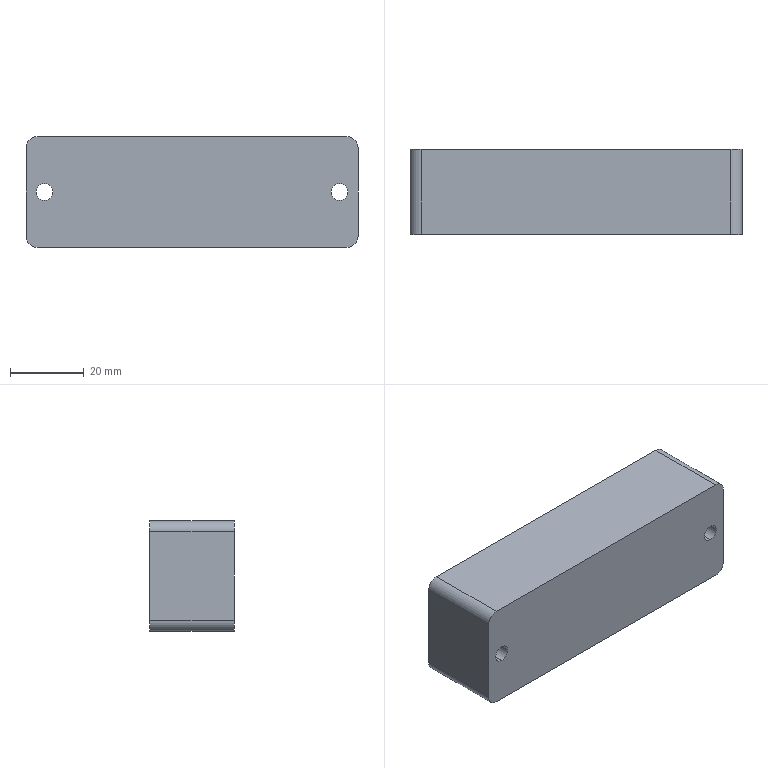Part | SolidWorks | features Extrusion 1, Fillet 1, HoleWzd 1 | 1 solid | 20 faces | box 90 x 23 x 30 mm | volume 60888 mm3 | cylinder 12 | plane 8 | commonest cylinder face diameters 4.5 x4 6 x4 8 x4
STEP:
#1=CARTESIAN_POINT('',(-40.,7.1,-4.));
#2=VERTEX_POINT('',#1);
#3=CARTESIAN_POINT('',(-40.,7.1,4.));
#4=VERTEX_POINT('',#3);
#5=CARTESIAN_POINT('',(-40.,7.1,0.));
#6=DIRECTION('',(0.,1.,0.));
#7=DIRECTION('',(0.,0.,1.));
#8=AXIS2_PLACEMENT_3D('',#5,#6,#7);
#9=CIRCLE('',#8,4.);
#10=EDGE_CURVE('',#2,#4,#9,.T.);
#11=ORIENTED_EDGE('',*,*,#10,.F.);
#12=CARTESIAN_POINT('',(-40.,11.5,-4.));
#13=VERTEX_POINT('',#12);
#14=CARTESIAN_POINT('',(-40.,11.5,-4.));
#15=DIRECTION('',(0.,1.,0.));
#16=VECTOR('',#15,1000.);
#17=LINE('',#14,#16);
#18=EDGE_CURVE('',#2,#13,#17,.T.);
#19=ORIENTED_EDGE('',*,*,#18,.T.);
#20=CARTESIAN_POINT('',(-40.,11.5,4.));
#21=VERTEX_POINT('',#20);
#22=CARTESIAN_POINT('',(-40.,11.5,0.));
#23=DIRECTION('',(0.,1.,0.));
#24=DIRECTION('',(0.,0.,1.));
#25=AXIS2_PLACEMENT_3D('',#22,#23,#24);
#26=CIRCLE('',#25,4.);
#27=EDGE_CURVE('',#13,#21,#26,.T.);
#28=ORIENTED_EDGE('',*,*,#27,.T.);
#29=CARTESIAN_POINT('',(-40.,11.5,4.));
#30=DIRECTION('',(0.,1.,0.));
#31=VECTOR('',#30,1000.);
#32=LINE('',#29,#31);
#33=EDGE_CURVE('',#4,#21,#32,.T.);
#34=ORIENTED_EDGE('',*,*,#33,.F.);
#35=EDGE_LOOP('',(#11,#19,#28,#34));
#36=FACE_OUTER_BOUND('',#35,.T.);
#37=CARTESIAN_POINT('',(-40.,11.5,0.));
#38=DIRECTION('',(0.,1.,0.));
#39=DIRECTION('',(0.,0.,1.));
#40=AXIS2_PLACEMENT_3D('',#37,#38,#39);
#41=CYLINDRICAL_SURFACE('',#40,4.);
#42=ADVANCED_FACE('',(#36),#41,.F.);
#43=CARTESIAN_POINT('',(-40.,-11.5,-2.25));
#44=VERTEX_POINT('',#43);
#45=CARTESIAN_POINT('',(-40.,-11.5,2.25));
#46=VERTEX_POINT('',#45);
#47=CARTESIAN_POINT('',(-40.,-11.5,0.));
#48=DIRECTION('',(0.,1.,0.));
#49=DIRECTION('',(0.,0.,1.));
#50=AXIS2_PLACEMENT_3D('',#47,#48,#49);
#51=CIRCLE('',#50,2.25);
#52=EDGE_CURVE('',#44,#46,#51,.T.);
#53=ORIENTED_EDGE('',*,*,#52,.F.);
#54=CARTESIAN_POINT('',(-40.,7.1,-2.25));
#55=VERTEX_POINT('',#54);
#56=CARTESIAN_POINT('',(-40.,11.5,-2.25));
#57=DIRECTION('',(0.,1.,0.));
#58=VECTOR('',#57,1000.);
#59=LINE('',#56,#58);
#60=EDGE_CURVE('',#44,#55,#59,.T.);
#61=ORIENTED_EDGE('',*,*,#60,.T.);
#62=CARTESIAN_POINT('',(-40.,7.1,2.25));
#63=VERTEX_POINT('',#62);
#64=CARTESIAN_POINT('',(-40.,7.1,0.));
#65=DIRECTION('',(0.,1.,0.));
#66=DIRECTION('',(0.,0.,1.));
#67=AXIS2_PLACEMENT_3D('',#64,#65,#66);
#68=CIRCLE('',#67,2.25);
#69=EDGE_CURVE('',#55,#63,#68,.T.);
#70=ORIENTED_EDGE('',*,*,#69,.T.);
#71=CARTESIAN_POINT('',(-40.,11.5,2.25));
#72=DIRECTION('',(0.,1.,0.));
#73=VECTOR('',#72,1000.);
#74=LINE('',#71,#73);
#75=EDGE_CURVE('',#46,#63,#74,.T.);
#76=ORIENTED_EDGE('',*,*,#75,.F.);
#77=EDGE_LOOP('',(#53,#61,#70,#76));
#78=FACE_OUTER_BOUND('',#77,.T.);
#79=CARTESIAN_POINT('',(-40.,11.5,0.));
#80=DIRECTION('',(0.,1.,0.));
#81=DIRECTION('',(0.,0.,1.));
#82=AXIS2_PLACEMENT_3D('',#79,#80,#81);
#83=CYLINDRICAL_SURFACE('',#82,2.25);
#84=ADVANCED_FACE('',(#78),#83,.F.);
#85=CARTESIAN_POINT('',(40.,7.1,-4.));
#86=VERTEX_POINT('',#85);
#87=CARTESIAN_POINT('',(40.,7.1,4.));
#88=VERTEX_POINT('',#87);
#89=CARTESIAN_POINT('',(40.,7.1,0.));
#90=DIRECTION('',(0.,1.,0.));
#91=DIRECTION('',(0.,0.,1.));
#92=AXIS2_PLACEMENT_3D('',#89,#90,#91);
#93=CIRCLE('',#92,4.);
#94=EDGE_CURVE('',#86,#88,#93,.T.);
#95=ORIENTED_EDGE('',*,*,#94,.F.);
#96=CARTESIAN_POINT('',(40.,11.5,-4.));
#97=VERTEX_POINT('',#96);
#98=CARTESIAN_POINT('',(40.,11.5,-4.));
#99=DIRECTION('',(0.,1.,0.));
#100=VECTOR('',#99,1000.);
#101=LINE('',#98,#100);
#102=EDGE_CURVE('',#86,#97,#101,.T.);
#103=ORIENTED_EDGE('',*,*,#102,.T.);
#104=CARTESIAN_POINT('',(40.,11.5,4.));
#105=VERTEX_POINT('',#104);
#106=CARTESIAN_POINT('',(40.,11.5,0.));
#107=DIRECTION('',(0.,1.,0.));
#108=DIRECTION('',(0.,0.,1.));
#109=AXIS2_PLACEMENT_3D('',#106,#107,#108);
#110=CIRCLE('',#109,4.);
#111=EDGE_CURVE('',#97,#105,#110,.T.);
#112=ORIENTED_EDGE('',*,*,#111,.T.);
#113=CARTESIAN_POINT('',(40.,11.5,4.));
#114=DIRECTION('',(0.,1.,0.));
#115=VECTOR('',#114,1000.);
#116=LINE('',#113,#115);
#117=EDGE_CURVE('',#88,#105,#116,.T.);
#118=ORIENTED_EDGE('',*,*,#117,.F.);
#119=EDGE_LOOP('',(#95,#103,#112,#118));
#120=FACE_OUTER_BOUND('',#119,.T.);
#121=CARTESIAN_POINT('',(40.,11.5,0.));
#122=DIRECTION('',(0.,1.,0.));
#123=DIRECTION('',(0.,0.,1.));
#124=AXIS2_PLACEMENT_3D('',#121,#122,#123);
#125=CYLINDRICAL_SURFACE('',#124,4.);
#126=ADVANCED_FACE('',(#120),#125,.F.);
#127=CARTESIAN_POINT('',(40.,-11.5,-2.25));
#128=VERTEX_POINT('',#127);
#129=CARTESIAN_POINT('',(40.,-11.5,2.25));
#130=VERTEX_POINT('',#129);
#131=CARTESIAN_POINT('',(40.,-11.5,0.));
#132=DIRECTION('',(0.,1.,0.));
#133=DIRECTION('',(0.,0.,1.));
#134=AXIS2_PLACEMENT_3D('',#131,#132,#133);
#135=CIRCLE('',#134,2.25);
#136=EDGE_CURVE('',#128,#130,#135,.T.);
#137=ORIENTED_EDGE('',*,*,#136,.F.);
#138=CARTESIAN_POINT('',(40.,7.1,-2.25));
#139=VERTEX_POINT('',#138);
#140=CARTESIAN_POINT('',(40.,11.5,-2.25));
#141=DIRECTION('',(0.,1.,0.));
#142=VECTOR('',#141,1000.);
#143=LINE('',#140,#142);
#144=EDGE_CURVE('',#128,#139,#143,.T.);
#145=ORIENTED_EDGE('',*,*,#144,.T.);
#146=CARTESIAN_POINT('',(40.,7.1,2.25));
#147=VERTEX_POINT('',#146);
#148=CARTESIAN_POINT('',(40.,7.1,0.));
#149=DIRECTION('',(0.,1.,0.));
#150=DIRECTION('',(0.,0.,1.));
#151=AXIS2_PLACEMENT_3D('',#148,#149,#150);
#152=CIRCLE('',#151,2.25);
#153=EDGE_CURVE('',#139,#147,#152,.T.);
#154=ORIENTED_EDGE('',*,*,#153,.T.);
#155=CARTESIAN_POINT('',(40.,11.5,2.25));
#156=DIRECTION('',(0.,1.,0.));
#157=VECTOR('',#156,1000.);
#158=LINE('',#155,#157);
#159=EDGE_CURVE('',#130,#147,#158,.T.);
#160=ORIENTED_EDGE('',*,*,#159,.F.);
#161=EDGE_LOOP('',(#137,#145,#154,#160));
#162=FACE_OUTER_BOUND('',#161,.T.);
#163=CARTESIAN_POINT('',(40.,11.5,0.));
#164=DIRECTION('',(0.,1.,0.));
#165=DIRECTION('',(0.,0.,1.));
#166=AXIS2_PLACEMENT_3D('',#163,#164,#165);
#167=CYLINDRICAL_SURFACE('',#166,2.25);
#168=ADVANCED_FACE('',(#162),#167,.F.);
#169=CARTESIAN_POINT('',(45.,11.5,12.));
#170=VERTEX_POINT('',#169);
#171=CARTESIAN_POINT('',(45.,11.5,-12.));
#172=VERTEX_POINT('',#171);
#173=CARTESIAN_POINT('',(45.,11.5,15.));
#174=DIRECTION('',(0.,0.,-1.));
#175=VECTOR('',#174,1000.);
#176=LINE('',#173,#175);
#177=EDGE_CURVE('',#170,#172,#176,.T.);
#178=ORIENTED_EDGE('',*,*,#177,.F.);
#179=CARTESIAN_POINT('',(45.,-11.5,12.));
#180=VERTEX_POINT('',#179);
#181=CARTESIAN_POINT('',(45.,11.5,12.));
#182=DIRECTION('',(0.,-1.,0.));
#183=VECTOR('',#182,1000.);
#184=LINE('',#181,#183);
#185=EDGE_CURVE('',#170,#180,#184,.T.);
#186=ORIENTED_EDGE('',*,*,#185,.T.);
#187=CARTESIAN_POINT('',(45.,-11.5,-12.));
#188=VERTEX_POINT('',#187);
#189=CARTESIAN_POINT('',(45.,-11.5,15.));
#190=DIRECTION('',(0.,0.,-1.));
#191=VECTOR('',#190,1000.);
#192=LINE('',#189,#191);
#193=EDGE_CURVE('',#180,#188,#192,.T.);
#194=ORIENTED_EDGE('',*,*,#193,.T.);
#195=CARTESIAN_POINT('',(45.,11.5,-12.));
#196=DIRECTION('',(0.,1.,0.));
#197=VECTOR('',#196,1000.);
#198=LINE('',#195,#197);
#199=EDGE_CURVE('',#188,#172,#198,.T.);
#200=ORIENTED_EDGE('',*,*,#199,.T.);
#201=EDGE_LOOP('',(#178,#186,#194,#200));
#202=FACE_OUTER_BOUND('',#201,.T.);
#203=CARTESIAN_POINT('',(45.,11.5,15.));
#204=DIRECTION('',(-1.,0.,0.));
#205=DIRECTION('',(0.,0.,1.));
#206=AXIS2_PLACEMENT_3D('',#203,#204,#205);
#207=PLANE('',#206);
#208=ADVANCED_FACE('',(#202),#207,.F.);
#209=CARTESIAN_POINT('',(42.,11.5,-15.));
#210=VERTEX_POINT('',#209);
#211=CARTESIAN_POINT('',(-42.,11.5,-15.));
#212=VERTEX_POINT('',#211);
#213=CARTESIAN_POINT('',(-45.,11.5,-15.));
#214=DIRECTION('',(-1.,0.,0.));
#215=VECTOR('',#214,1000.);
#216=LINE('',#213,#215);
#217=EDGE_CURVE('',#210,#212,#216,.T.);
#218=ORIENTED_EDGE('',*,*,#217,.F.);
#219=CARTESIAN_POINT('',(42.,-11.5,-15.));
#220=VERTEX_POINT('',#219);
#221=CARTESIAN_POINT('',(42.,11.5,-15.));
#222=DIRECTION('',(0.,-1.,0.));
#223=VECTOR('',#222,1000.);
#224=LINE('',#221,#223);
#225=EDGE_CURVE('',#210,#220,#224,.T.);
#226=ORIENTED_EDGE('',*,*,#225,.T.);
#227=CARTESIAN_POINT('',(-42.,-11.5,-15.));
#228=VERTEX_POINT('',#227);
#229=CARTESIAN_POINT('',(-45.,-11.5,-15.));
#230=DIRECTION('',(-1.,0.,0.));
#231=VECTOR('',#230,1000.);
#232=LINE('',#229,#231);
#233=EDGE_CURVE('',#220,#228,#232,.T.);
#234=ORIENTED_EDGE('',*,*,#233,.T.);
#235=CARTESIAN_POINT('',(-42.,11.5,-15.));
#236=DIRECTION('',(0.,1.,0.));
#237=VECTOR('',#236,1000.);
#238=LINE('',#235,#237);
#239=EDGE_CURVE('',#228,#212,#238,.T.);
#240=ORIENTED_EDGE('',*,*,#239,.T.);
#241=EDGE_LOOP('',(#218,#226,#234,#240));
#242=FACE_OUTER_BOUND('',#241,.T.);
#243=CARTESIAN_POINT('',(-45.,11.5,-15.));
#244=DIRECTION('',(0.,0.,1.));
#245=DIRECTION('',(1.,0.,0.));
#246=AXIS2_PLACEMENT_3D('',#243,#244,#245);
#247=PLANE('',#246);
#248=ADVANCED_FACE('',(#242),#247,.F.);
#249=CARTESIAN_POINT('',(-45.,11.5,-12.));
#250=VERTEX_POINT('',#249);
#251=CARTESIAN_POINT('',(-45.,11.5,12.));
#252=VERTEX_POINT('',#251);
#253=CARTESIAN_POINT('',(-45.,11.5,15.));
#254=DIRECTION('',(0.,0.,1.));
#255=VECTOR('',#254,1000.);
#256=LINE('',#253,#255);
#257=EDGE_CURVE('',#250,#252,#256,.T.);
#258=ORIENTED_EDGE('',*,*,#257,.F.);
#259=CARTESIAN_POINT('',(-45.,-11.5,-12.));
#260=VERTEX_POINT('',#259);
#261=CARTESIAN_POINT('',(-45.,11.5,-12.));
#262=DIRECTION('',(0.,-1.,0.));
#263=VECTOR('',#262,1000.);
#264=LINE('',#261,#263);
#265=EDGE_CURVE('',#250,#260,#264,.T.);
#266=ORIENTED_EDGE('',*,*,#265,.T.);
#267=CARTESIAN_POINT('',(-45.,-11.5,12.));
#268=VERTEX_POINT('',#267);
#269=CARTESIAN_POINT('',(-45.,-11.5,15.));
#270=DIRECTION('',(0.,0.,1.));
#271=VECTOR('',#270,1000.);
#272=LINE('',#269,#271);
#273=EDGE_CURVE('',#260,#268,#272,.T.);
#274=ORIENTED_EDGE('',*,*,#273,.T.);
#275=CARTESIAN_POINT('',(-45.,11.5,12.));
#276=DIRECTION('',(0.,1.,0.));
#277=VECTOR('',#276,1000.);
#278=LINE('',#275,#277);
#279=EDGE_CURVE('',#268,#252,#278,.T.);
#280=ORIENTED_EDGE('',*,*,#279,.T.);
#281=EDGE_LOOP('',(#258,#266,#274,#280));
#282=FACE_OUTER_BOUND('',#281,.T.);
#283=CARTESIAN_POINT('',(-45.,11.5,15.));
#284=DIRECTION('',(1.,0.,0.));
#285=DIRECTION('',(0.,0.,-1.));
#286=AXIS2_PLACEMENT_3D('',#283,#284,#285);
#287=PLANE('',#286);
#288=ADVANCED_FACE('',(#282),#287,.F.);
#289=CARTESIAN_POINT('',(-42.,-11.5,15.));
#290=VERTEX_POINT('',#289);
#291=CARTESIAN_POINT('',(42.,-11.5,15.));
#292=VERTEX_POINT('',#291);
#293=CARTESIAN_POINT('',(-45.,-11.5,15.));
#294=DIRECTION('',(1.,0.,0.));
#295=VECTOR('',#294,1000.);
#296=LINE('',#293,#295);
#297=EDGE_CURVE('',#290,#292,#296,.T.);
#298=ORIENTED_EDGE('',*,*,#297,.T.);
#299=CARTESIAN_POINT('',(42.,11.5,15.));
#300=VERTEX_POINT('',#299);
#301=CARTESIAN_POINT('',(42.,11.5,15.));
#302=DIRECTION('',(0.,1.,0.));
#303=VECTOR('',#302,1000.);
#304=LINE('',#301,#303);
#305=EDGE_CURVE('',#292,#300,#304,.T.);
#306=ORIENTED_EDGE('',*,*,#305,.T.);
#307=CARTESIAN_POINT('',(-42.,11.5,15.));
#308=VERTEX_POINT('',#307);
#309=CARTESIAN_POINT('',(-45.,11.5,15.));
#310=DIRECTION('',(1.,0.,0.));
#311=VECTOR('',#310,1000.);
#312=LINE('',#309,#311);
#313=EDGE_CURVE('',#308,#300,#312,.T.);
#314=ORIENTED_EDGE('',*,*,#313,.F.);
#315=CARTESIAN_POINT('',(-42.,11.5,15.));
#316=DIRECTION('',(0.,-1.,0.));
#317=VECTOR('',#316,1000.);
#318=LINE('',#315,#317);
#319=EDGE_CURVE('',#308,#290,#318,.T.);
#320=ORIENTED_EDGE('',*,*,#319,.T.);
#321=EDGE_LOOP('',(#298,#306,#314,#320));
#322=FACE_OUTER_BOUND('',#321,.T.);
#323=CARTESIAN_POINT('',(-45.,11.5,15.));
#324=DIRECTION('',(0.,0.,-1.));
#325=DIRECTION('',(-1.,0.,0.));
#326=AXIS2_PLACEMENT_3D('',#323,#324,#325);
#327=PLANE('',#326);
#328=ADVANCED_FACE('',(#322),#327,.F.);
#329=CARTESIAN_POINT('',(-40.,11.5,0.));
#330=DIRECTION('',(0.,1.,0.));
#331=DIRECTION('',(0.,0.,1.));
#332=AXIS2_PLACEMENT_3D('',#329,#330,#331);
#333=CIRCLE('',#332,4.);
#334=EDGE_CURVE('',#21,#13,#333,.T.);
#335=ORIENTED_EDGE('',*,*,#334,.F.);
#336=ORIENTED_EDGE('',*,*,#27,.F.);
#337=EDGE_LOOP('',(#335,#336));
#338=FACE_BOUND('',#337,.T.);
#339=CARTESIAN_POINT('',(40.,11.5,0.));
#340=DIRECTION('',(0.,1.,0.));
#341=DIRECTION('',(0.,0.,1.));
#342=AXIS2_PLACEMENT_3D('',#339,#340,#341);
#343=CIRCLE('',#342,4.);
#344=EDGE_CURVE('',#105,#97,#343,.T.);
#345=ORIENTED_EDGE('',*,*,#344,.F.);
#346=ORIENTED_EDGE('',*,*,#111,.F.);
#347=EDGE_LOOP('',(#345,#346));
#348=FACE_BOUND('',#347,.T.);
#349=ORIENTED_EDGE('',*,*,#313,.T.);
#350=CARTESIAN_POINT('',(42.,11.5,12.));
#351=DIRECTION('',(0.,1.,0.));
#352=DIRECTION('',(0.,0.,-1.));
#353=AXIS2_PLACEMENT_3D('',#350,#351,#352);
#354=CIRCLE('',#353,3.);
#355=EDGE_CURVE('',#300,#170,#354,.T.);
#356=ORIENTED_EDGE('',*,*,#355,.T.);
#357=ORIENTED_EDGE('',*,*,#177,.T.);
#358=CARTESIAN_POINT('',(42.,11.5,-12.));
#359=DIRECTION('',(0.,1.,0.));
#360=DIRECTION('',(0.,0.,-1.));
#361=AXIS2_PLACEMENT_3D('',#358,#359,#360);
#362=CIRCLE('',#361,3.);
#363=EDGE_CURVE('',#172,#210,#362,.T.);
#364=ORIENTED_EDGE('',*,*,#363,.T.);
#365=ORIENTED_EDGE('',*,*,#217,.T.);
#366=CARTESIAN_POINT('',(-42.,11.5,-12.));
#367=DIRECTION('',(0.,1.,0.));
#368=DIRECTION('',(0.,0.,-1.));
#369=AXIS2_PLACEMENT_3D('',#366,#367,#368);
#370=CIRCLE('',#369,3.);
#371=EDGE_CURVE('',#212,#250,#370,.T.);
#372=ORIENTED_EDGE('',*,*,#371,.T.);
#373=ORIENTED_EDGE('',*,*,#257,.T.);
#374=CARTESIAN_POINT('',(-42.,11.5,12.));
#375=DIRECTION('',(0.,1.,0.));
#376=DIRECTION('',(0.,0.,-1.));
#377=AXIS2_PLACEMENT_3D('',#374,#375,#376);
#378=CIRCLE('',#377,3.);
#379=EDGE_CURVE('',#252,#308,#378,.T.);
#380=ORIENTED_EDGE('',*,*,#379,.T.);
#381=EDGE_LOOP('',(#349,#356,#357,#364,#365,#372,#373,#380));
#382=FACE_OUTER_BOUND('',#381,.T.);
#383=CARTESIAN_POINT('',(0.,11.5,0.));
#384=DIRECTION('',(0.,-1.,0.));
#385=DIRECTION('',(0.,0.,-1.));
#386=AXIS2_PLACEMENT_3D('',#383,#384,#385);
#387=PLANE('',#386);
#388=ADVANCED_FACE('',(#338,#348,#382),#387,.F.);
#389=CARTESIAN_POINT('',(-40.,-11.5,0.));
#390=DIRECTION('',(0.,1.,0.));
#391=DIRECTION('',(0.,0.,1.));
#392=AXIS2_PLACEMENT_3D('',#389,#390,#391);
#393=CIRCLE('',#392,2.25);
#394=EDGE_CURVE('',#46,#44,#393,.T.);
#395=ORIENTED_EDGE('',*,*,#394,.T.);
#396=ORIENTED_EDGE('',*,*,#52,.T.);
#397=EDGE_LOOP('',(#395,#396));
#398=FACE_BOUND('',#397,.T.);
#399=CARTESIAN_POINT('',(40.,-11.5,0.));
#400=DIRECTION('',(0.,1.,0.));
#401=DIRECTION('',(0.,0.,1.));
#402=AXIS2_PLACEMENT_3D('',#399,#400,#401);
#403=CIRCLE('',#402,2.25);
#404=EDGE_CURVE('',#130,#128,#403,.T.);
#405=ORIENTED_EDGE('',*,*,#404,.T.);
#406=ORIENTED_EDGE('',*,*,#136,.T.);
#407=EDGE_LOOP('',(#405,#406));
#408=FACE_BOUND('',#407,.T.);
#409=ORIENTED_EDGE('',*,*,#193,.F.);
#410=CARTESIAN_POINT('',(42.,-11.5,12.));
#411=DIRECTION('',(0.,-1.,0.));
#412=DIRECTION('',(0.,0.,-1.));
#413=AXIS2_PLACEMENT_3D('',#410,#411,#412);
#414=CIRCLE('',#413,3.);
#415=EDGE_CURVE('',#180,#292,#414,.T.);
#416=ORIENTED_EDGE('',*,*,#415,.T.);
#417=ORIENTED_EDGE('',*,*,#297,.F.);
#418=CARTESIAN_POINT('',(-42.,-11.5,12.));
#419=DIRECTION('',(0.,-1.,0.));
#420=DIRECTION('',(0.,0.,-1.));
#421=AXIS2_PLACEMENT_3D('',#418,#419,#420);
#422=CIRCLE('',#421,3.);
#423=EDGE_CURVE('',#290,#268,#422,.T.);
#424=ORIENTED_EDGE('',*,*,#423,.T.);
#425=ORIENTED_EDGE('',*,*,#273,.F.);
#426=CARTESIAN_POINT('',(-42.,-11.5,-12.));
#427=DIRECTION('',(0.,-1.,0.));
#428=DIRECTION('',(0.,0.,-1.));
#429=AXIS2_PLACEMENT_3D('',#426,#427,#428);
#430=CIRCLE('',#429,3.);
#431=EDGE_CURVE('',#260,#228,#430,.T.);
#432=ORIENTED_EDGE('',*,*,#431,.T.);
#433=ORIENTED_EDGE('',*,*,#233,.F.);
#434=CARTESIAN_POINT('',(42.,-11.5,-12.));
#435=DIRECTION('',(0.,-1.,0.));
#436=DIRECTION('',(0.,0.,-1.));
#437=AXIS2_PLACEMENT_3D('',#434,#435,#436);
#438=CIRCLE('',#437,3.);
#439=EDGE_CURVE('',#220,#188,#438,.T.);
#440=ORIENTED_EDGE('',*,*,#439,.T.);
#441=EDGE_LOOP('',(#409,#416,#417,#424,#425,#432,#433,#440));
#442=FACE_OUTER_BOUND('',#441,.T.);
#443=CARTESIAN_POINT('',(0.,-11.5,0.));
#444=DIRECTION('',(0.,-1.,0.));
#445=DIRECTION('',(0.,0.,-1.));
#446=AXIS2_PLACEMENT_3D('',#443,#444,#445);
#447=PLANE('',#446);
#448=ADVANCED_FACE('',(#398,#408,#442),#447,.T.);
#449=ORIENTED_EDGE('',*,*,#144,.F.);
#450=ORIENTED_EDGE('',*,*,#404,.F.);
#451=ORIENTED_EDGE('',*,*,#159,.T.);
#452=CARTESIAN_POINT('',(40.,7.1,0.));
#453=DIRECTION('',(0.,1.,0.));
#454=DIRECTION('',(0.,0.,1.));
#455=AXIS2_PLACEMENT_3D('',#452,#453,#454);
#456=CIRCLE('',#455,2.25);
#457=EDGE_CURVE('',#147,#139,#456,.T.);
#458=ORIENTED_EDGE('',*,*,#457,.T.);
#459=EDGE_LOOP('',(#449,#450,#451,#458));
#460=FACE_OUTER_BOUND('',#459,.T.);
#461=CARTESIAN_POINT('',(40.,11.5,0.));
#462=DIRECTION('',(0.,1.,0.));
#463=DIRECTION('',(0.,0.,1.));
#464=AXIS2_PLACEMENT_3D('',#461,#462,#463);
#465=CYLINDRICAL_SURFACE('',#464,2.25);
#466=ADVANCED_FACE('',(#460),#465,.F.);
#467=ORIENTED_EDGE('',*,*,#457,.F.);
#468=ORIENTED_EDGE('',*,*,#153,.F.);
#469=EDGE_LOOP('',(#467,#468));
#470=FACE_BOUND('',#469,.T.);
#471=CARTESIAN_POINT('',(40.,7.1,0.));
#472=DIRECTION('',(0.,1.,0.));
#473=DIRECTION('',(0.,0.,1.));
#474=AXIS2_PLACEMENT_3D('',#471,#472,#473);
#475=CIRCLE('',#474,4.);
#476=EDGE_CURVE('',#88,#86,#475,.T.);
#477=ORIENTED_EDGE('',*,*,#476,.T.);
#478=ORIENTED_EDGE('',*,*,#94,.T.);
#479=EDGE_LOOP('',(#477,#478));
#480=FACE_OUTER_BOUND('',#479,.T.);
#481=CARTESIAN_POINT('',(42.25,7.1,0.));
#482=DIRECTION('',(0.,-1.,0.));
#483=DIRECTION('',(0.,0.,-1.));
#484=AXIS2_PLACEMENT_3D('',#481,#482,#483);
#485=PLANE('',#484);
#486=ADVANCED_FACE('',(#470,#480),#485,.F.);
#487=ORIENTED_EDGE('',*,*,#102,.F.);
#488=ORIENTED_EDGE('',*,*,#476,.F.);
#489=ORIENTED_EDGE('',*,*,#117,.T.);
#490=ORIENTED_EDGE('',*,*,#344,.T.);
#491=EDGE_LOOP('',(#487,#488,#489,#490));
#492=FACE_OUTER_BOUND('',#491,.T.);
#493=CARTESIAN_POINT('',(40.,11.5,0.));
#494=DIRECTION('',(0.,1.,0.));
#495=DIRECTION('',(0.,0.,1.));
#496=AXIS2_PLACEMENT_3D('',#493,#494,#495);
#497=CYLINDRICAL_SURFACE('',#496,4.);
#498=ADVANCED_FACE('',(#492),#497,.F.);
#499=ORIENTED_EDGE('',*,*,#60,.F.);
#500=ORIENTED_EDGE('',*,*,#394,.F.);
#501=ORIENTED_EDGE('',*,*,#75,.T.);
#502=CARTESIAN_POINT('',(-40.,7.1,0.));
#503=DIRECTION('',(0.,1.,0.));
#504=DIRECTION('',(0.,0.,1.));
#505=AXIS2_PLACEMENT_3D('',#502,#503,#504);
#506=CIRCLE('',#505,2.25);
#507=EDGE_CURVE('',#63,#55,#506,.T.);
#508=ORIENTED_EDGE('',*,*,#507,.T.);
#509=EDGE_LOOP('',(#499,#500,#501,#508));
#510=FACE_OUTER_BOUND('',#509,.T.);
#511=CARTESIAN_POINT('',(-40.,11.5,0.));
#512=DIRECTION('',(0.,1.,0.));
#513=DIRECTION('',(0.,0.,1.));
#514=AXIS2_PLACEMENT_3D('',#511,#512,#513);
#515=CYLINDRICAL_SURFACE('',#514,2.25);
#516=ADVANCED_FACE('',(#510),#515,.F.);
#517=ORIENTED_EDGE('',*,*,#507,.F.);
#518=ORIENTED_EDGE('',*,*,#69,.F.);
#519=EDGE_LOOP('',(#517,#518));
#520=FACE_BOUND('',#519,.T.);
#521=CARTESIAN_POINT('',(-40.,7.1,0.));
#522=DIRECTION('',(0.,1.,0.));
#523=DIRECTION('',(0.,0.,1.));
#524=AXIS2_PLACEMENT_3D('',#521,#522,#523);
#525=CIRCLE('',#524,4.);
#526=EDGE_CURVE('',#4,#2,#525,.T.);
#527=ORIENTED_EDGE('',*,*,#526,.T.);
#528=ORIENTED_EDGE('',*,*,#10,.T.);
#529=EDGE_LOOP('',(#527,#528));
#530=FACE_OUTER_BOUND('',#529,.T.);
#531=CARTESIAN_POINT('',(-37.75,7.1,0.));
#532=DIRECTION('',(0.,-1.,0.));
#533=DIRECTION('',(0.,0.,-1.));
#534=AXIS2_PLACEMENT_3D('',#531,#532,#533);
#535=PLANE('',#534);
#536=ADVANCED_FACE('',(#520,#530),#535,.F.);
#537=ORIENTED_EDGE('',*,*,#18,.F.);
#538=ORIENTED_EDGE('',*,*,#526,.F.);
#539=ORIENTED_EDGE('',*,*,#33,.T.);
#540=ORIENTED_EDGE('',*,*,#334,.T.);
#541=EDGE_LOOP('',(#537,#538,#539,#540));
#542=FACE_OUTER_BOUND('',#541,.T.);
#543=CARTESIAN_POINT('',(-40.,11.5,0.));
#544=DIRECTION('',(0.,1.,0.));
#545=DIRECTION('',(0.,0.,1.));
#546=AXIS2_PLACEMENT_3D('',#543,#544,#545);
#547=CYLINDRICAL_SURFACE('',#546,4.);
#548=ADVANCED_FACE('',(#542),#547,.F.);
#549=ORIENTED_EDGE('',*,*,#355,.F.);
#550=ORIENTED_EDGE('',*,*,#305,.F.);
#551=ORIENTED_EDGE('',*,*,#415,.F.);
#552=ORIENTED_EDGE('',*,*,#185,.F.);
#553=EDGE_LOOP('',(#549,#550,#551,#552));
#554=FACE_OUTER_BOUND('',#553,.T.);
#555=CARTESIAN_POINT('',(42.,11.5,12.));
#556=DIRECTION('',(0.,-1.,0.));
#557=DIRECTION('',(0.,0.,-1.));
#558=AXIS2_PLACEMENT_3D('',#555,#556,#557);
#559=CYLINDRICAL_SURFACE('',#558,3.);
#560=ADVANCED_FACE('',(#554),#559,.T.);
#561=ORIENTED_EDGE('',*,*,#363,.F.);
#562=ORIENTED_EDGE('',*,*,#199,.F.);
#563=ORIENTED_EDGE('',*,*,#439,.F.);
#564=ORIENTED_EDGE('',*,*,#225,.F.);
#565=EDGE_LOOP('',(#561,#562,#563,#564));
#566=FACE_OUTER_BOUND('',#565,.T.);
#567=CARTESIAN_POINT('',(42.,11.5,-12.));
#568=DIRECTION('',(0.,-1.,0.));
#569=DIRECTION('',(0.,0.,-1.));
#570=AXIS2_PLACEMENT_3D('',#567,#568,#569);
#571=CYLINDRICAL_SURFACE('',#570,3.);
#572=ADVANCED_FACE('',(#566),#571,.T.);
#573=ORIENTED_EDGE('',*,*,#371,.F.);
#574=ORIENTED_EDGE('',*,*,#239,.F.);
#575=ORIENTED_EDGE('',*,*,#431,.F.);
#576=ORIENTED_EDGE('',*,*,#265,.F.);
#577=EDGE_LOOP('',(#573,#574,#575,#576));
#578=FACE_OUTER_BOUND('',#577,.T.);
#579=CARTESIAN_POINT('',(-42.,11.5,-12.));
#580=DIRECTION('',(0.,-1.,0.));
#581=DIRECTION('',(0.,0.,-1.));
#582=AXIS2_PLACEMENT_3D('',#579,#580,#581);
#583=CYLINDRICAL_SURFACE('',#582,3.);
#584=ADVANCED_FACE('',(#578),#583,.T.);
#585=ORIENTED_EDGE('',*,*,#379,.F.);
#586=ORIENTED_EDGE('',*,*,#279,.F.);
#587=ORIENTED_EDGE('',*,*,#423,.F.);
#588=ORIENTED_EDGE('',*,*,#319,.F.);
#589=EDGE_LOOP('',(#585,#586,#587,#588));
#590=FACE_OUTER_BOUND('',#589,.T.);
#591=CARTESIAN_POINT('',(-42.,11.5,12.));
#592=DIRECTION('',(0.,-1.,0.));
#593=DIRECTION('',(0.,0.,-1.));
#594=AXIS2_PLACEMENT_3D('',#591,#592,#593);
#595=CYLINDRICAL_SURFACE('',#594,3.);
#596=ADVANCED_FACE('',(#590),#595,.T.);
#597=CLOSED_SHELL('',(#42,#84,#126,#168,#208,#248,#288,#328,#388,#448,#466,#486,#498,#516,#536,#548,#560,#572,#584,#596));
#598=MANIFOLD_SOLID_BREP('',#597);
#599=CARTESIAN_POINT('',(0.,0.,0.));
#600=DIRECTION('',(0.,0.,1.));
#601=DIRECTION('',(1.,0.,0.));
#602=AXIS2_PLACEMENT_3D('',#599,#600,#601);
#603=(LENGTH_UNIT()NAMED_UNIT(*)SI_UNIT(.MILLI.,.METRE.));
#604=UNCERTAINTY_MEASURE_WITH_UNIT(LENGTH_MEASURE(0.00001),#603,'','');
#605=(NAMED_UNIT(*)PLANE_ANGLE_UNIT()SI_UNIT($,.RADIAN.));
#606=(NAMED_UNIT(*)SI_UNIT($,.STERADIAN.)SOLID_ANGLE_UNIT());
#607=(GEOMETRIC_REPRESENTATION_CONTEXT(3)GLOBAL_UNCERTAINTY_ASSIGNED_CONTEXT((#604))GLOBAL_UNIT_ASSIGNED_CONTEXT((#603,#605,#606))REPRESENTATION_CONTEXT('',''));
#608=ADVANCED_BREP_SHAPE_REPRESENTATION('',(#598,#602),#607);